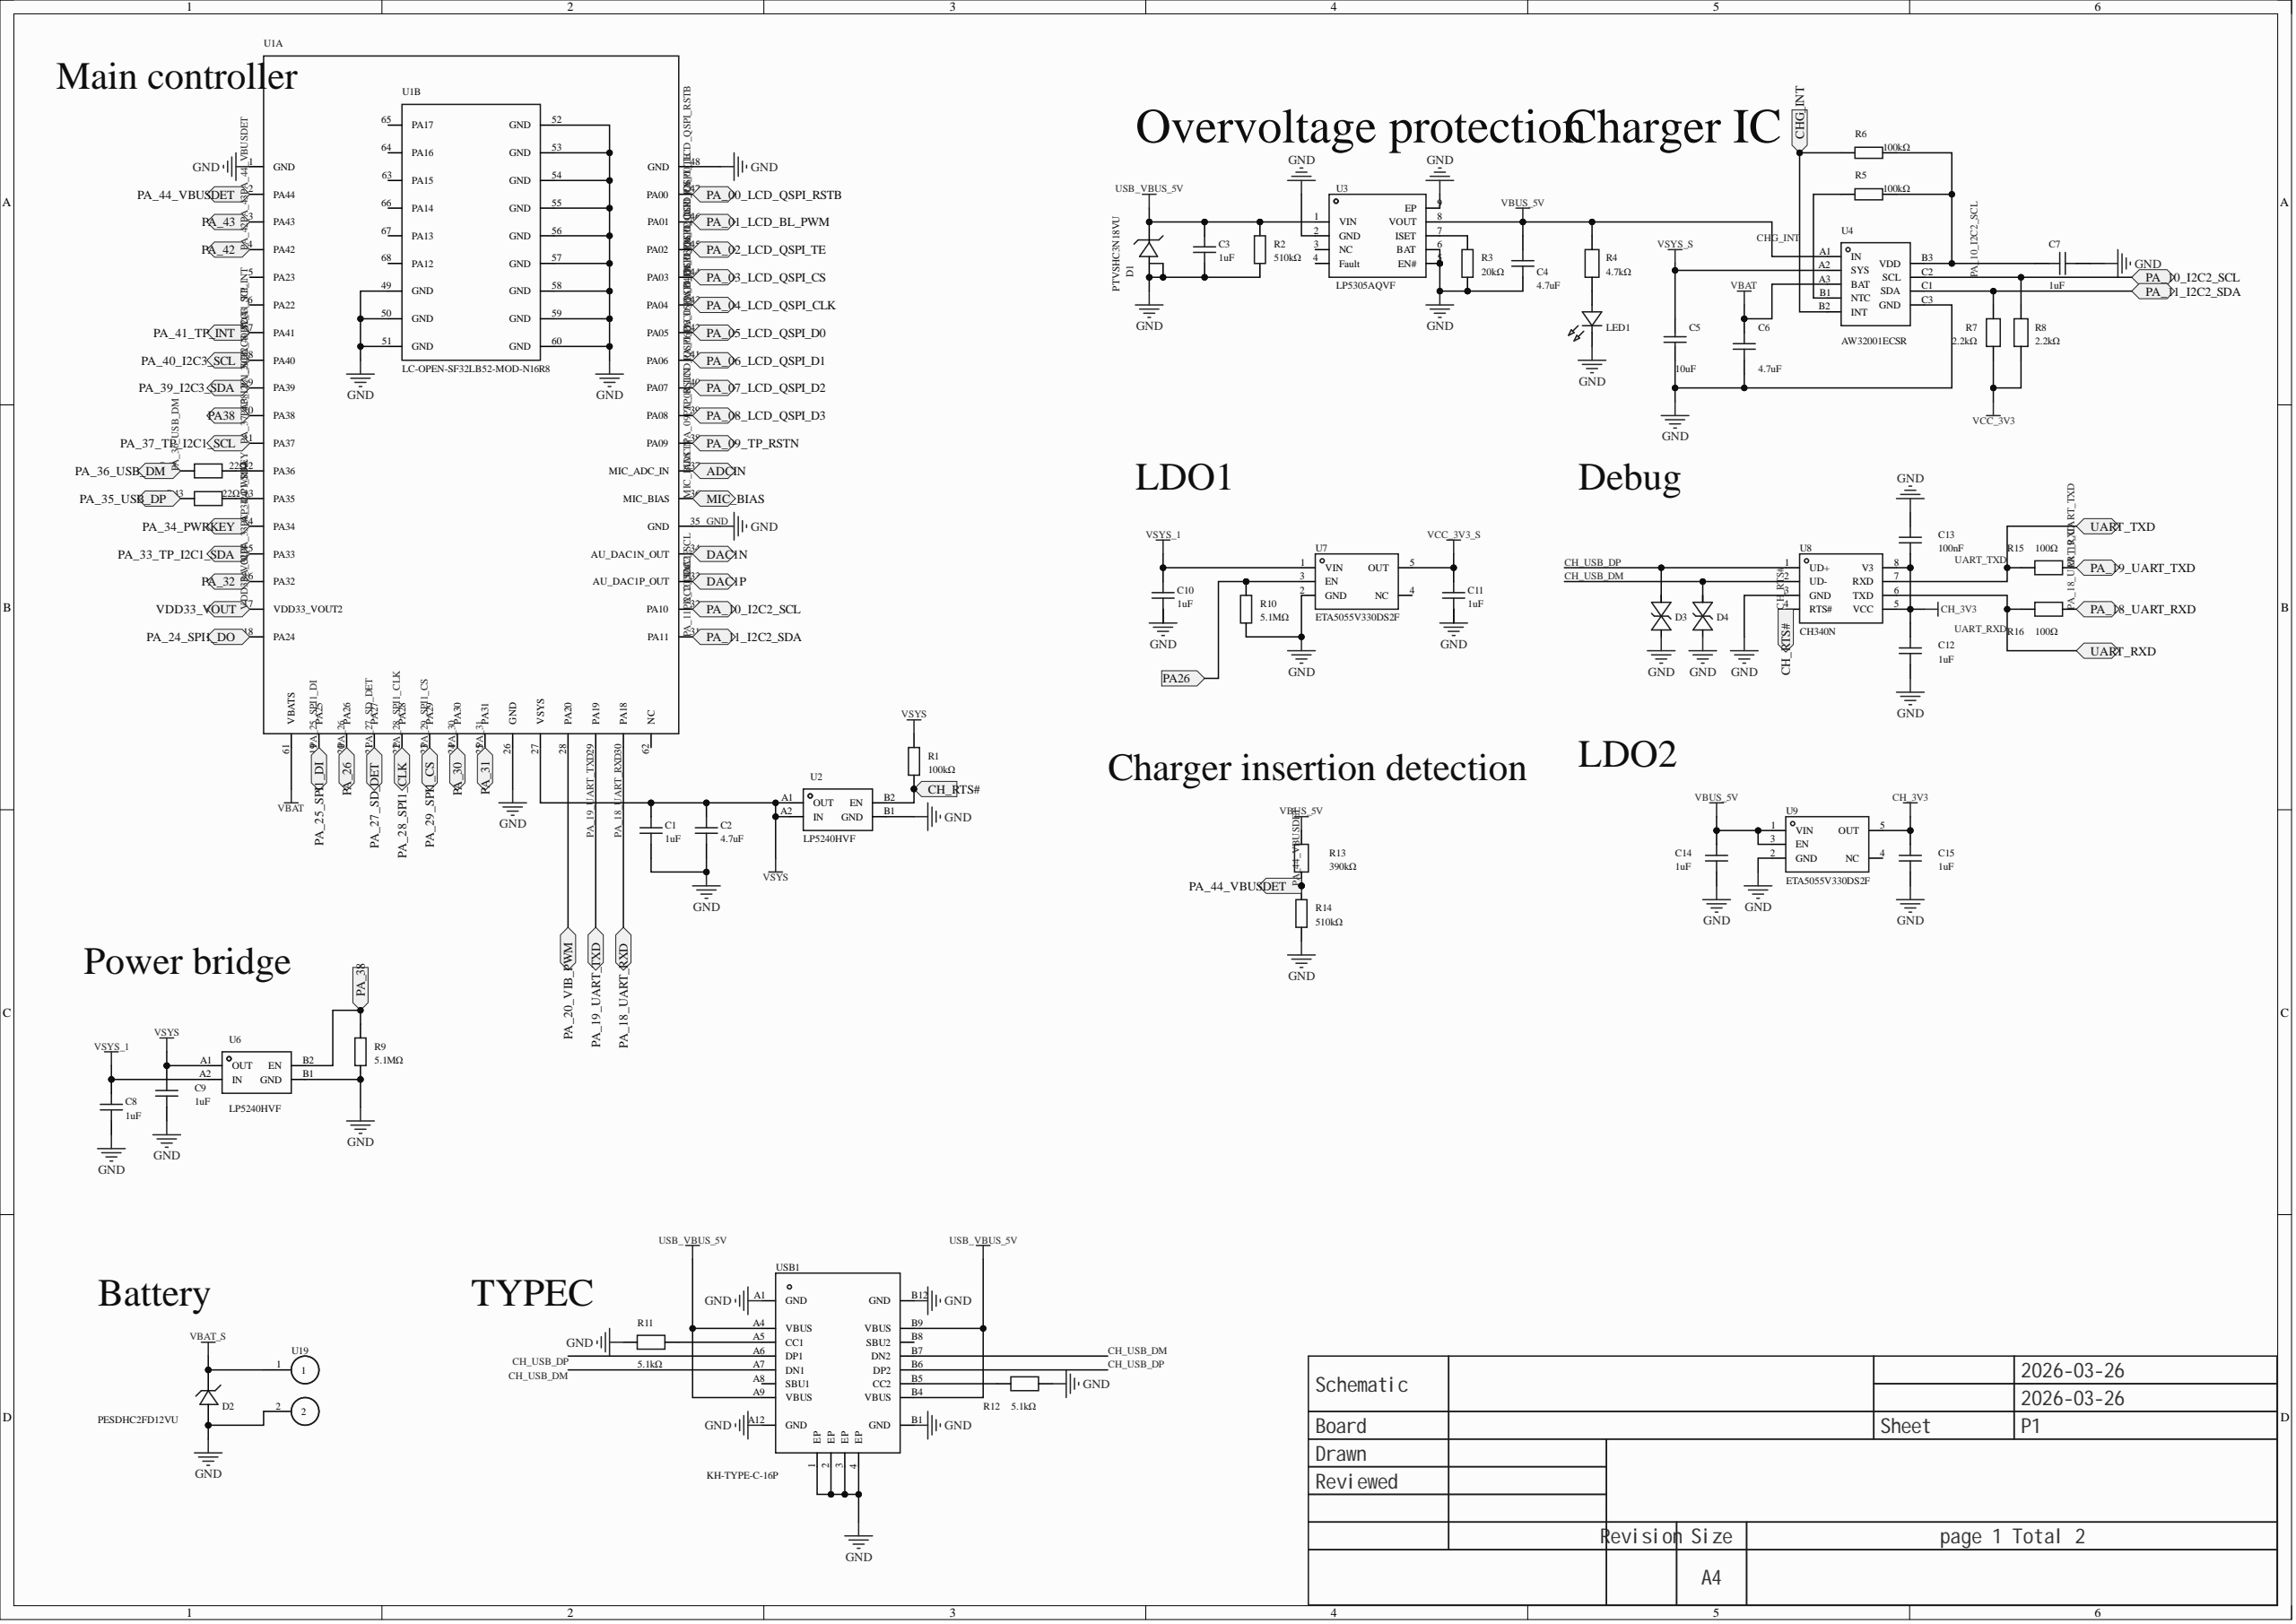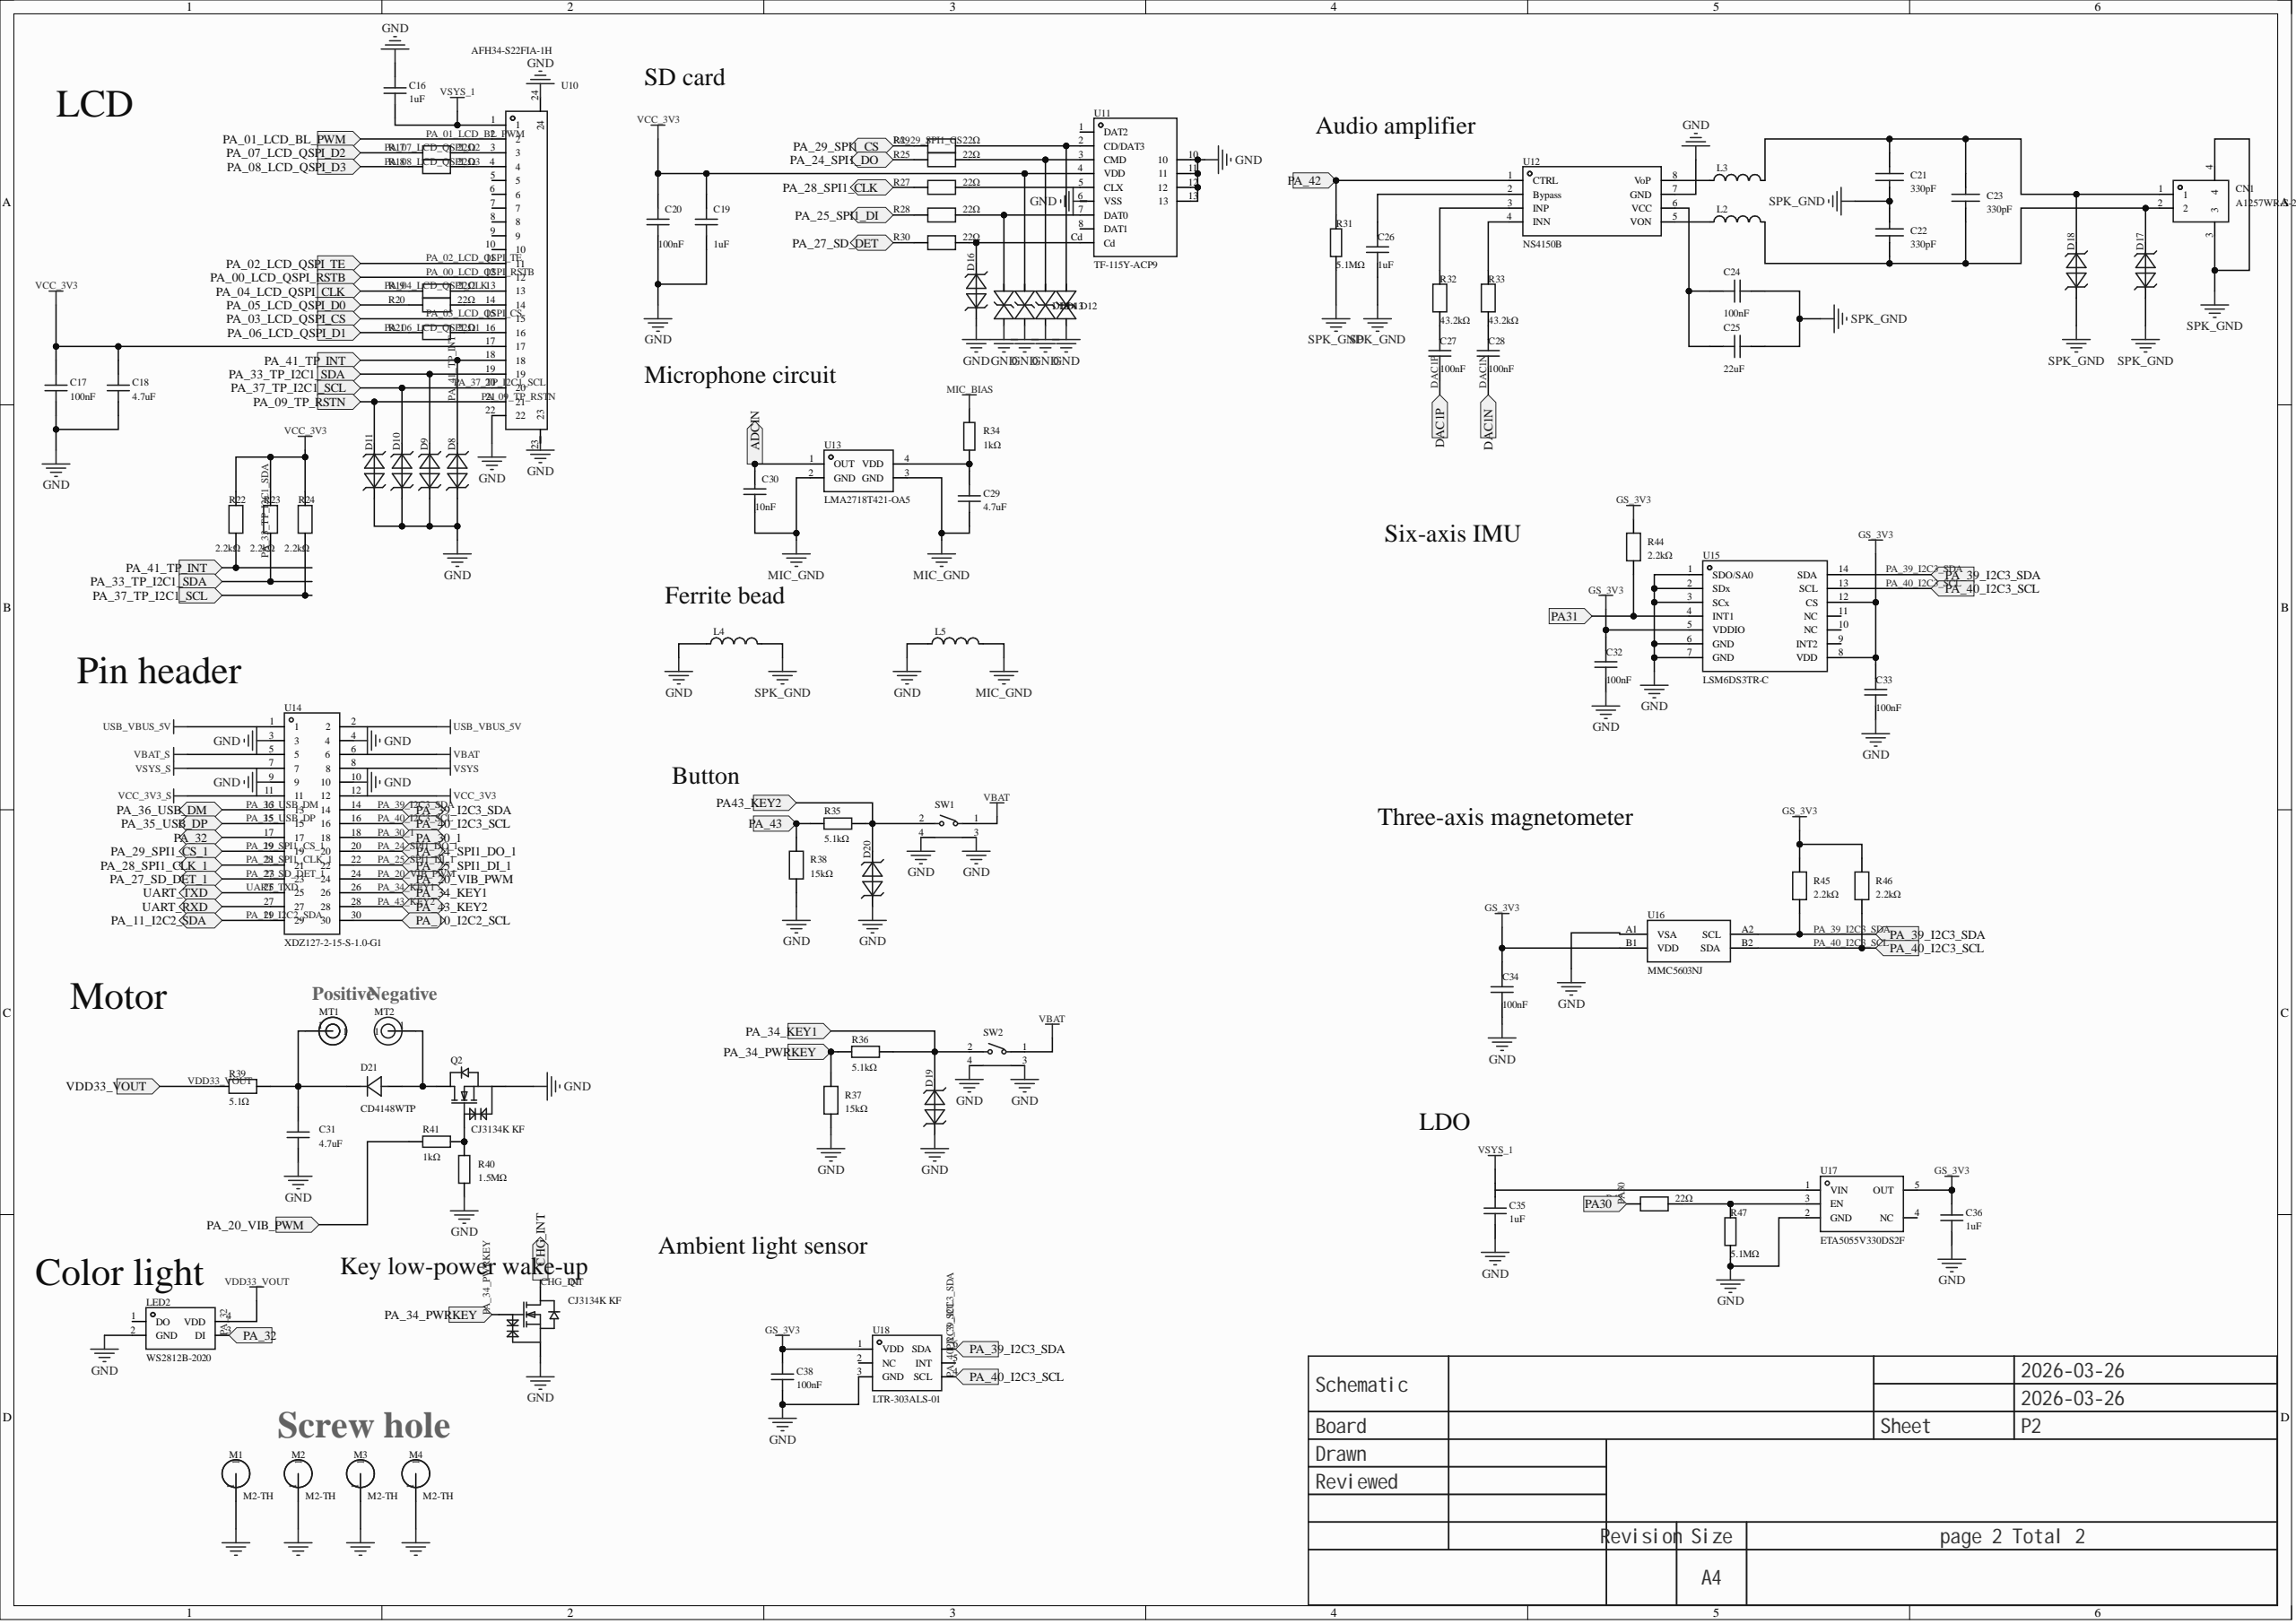Circuit board | Altium Designer | 138 parts | 94 nets
Bill of materials:
Comment,Description,Designator,Footprint,LibRef,Quantity
"1uF","Capacitance:1uF;Tolerance:±10%;Rated voltage:25V;Temperature coefficient:X5R;","C1, C3, C7, C8, C9, C10, C11, C12, C14, C15, C16, C19, C26, C35, C36","C0402","CL05A105KA5NQNC","15"
"4.7uF","Capacitance:4.7uF;Tolerance:±20%;Rated voltage:10V;Temperature coefficient:X5R;","C2, C4, C6, C18, C29, C31","C0402","CL05A475MP5NRNC","6"
"10uF","Capacitance:10uF;Tolerance:±20%;Rated voltage:6.3V;Temperature coefficient:X5R;","C5","C0402","CL05A106MQ5NUNC","1"
"100nF","Capacitance:100nF;Tolerance:±10%;Rated voltage:16V;Temperature coefficient:X7R;","C13, C17, C20, C24, C27, C28, C32, C33, C34, C38","C0402","CL05B104KO5NNNC","10"
"330pF","Capacitance:330pF;Tolerance:±5%;Rated voltage:50V;Temperature coefficient:C0G;","C21, C22, C23","C0402","CL05C331JB5NNNC","3"
"22uF","Capacitance:22uF;Tolerance:±20%;Rated voltage:6.3V;Temperature coefficient:X5R;","C25","C0402","GRM155R60J226ME11D","1"
"10nF","Capacitance:10nF;Tolerance:±10%;Rated voltage:50V;Temperature coefficient:X7R;","C30","C0402","CL05B103KB5NNNC","1"
"A1257WR-S-2P","Pin structure:1x2P;Pitch:1.25mm;Mounting:Horizontal;Reference series:GH;Total pins:2P;Rows:1;Pins per row:2;Row spacing:-;Rated current:1A;Contact material:Phosphor bronze;Contact plating:Tin;Operating temperature:-40℃~+105℃;","CN1","CONN-SMD_A1257WR-S-2P","A1257WR-S-2P","1"
"PTVSHC3N18VU","Reverse standoff voltage (Vrwm):18V;Clamping voltage:33V;Peak pulse current (Ipp):138A@8/20us;Peak pulse power (Ppp):4kW@8/20us;Breakdown voltage:20V;","D1","DFN-3_L2.0-W2.0-P1.30-BR","PTVSHC3N18VU","1"
"PESDHC2FD12VU","","D2","DFN1006-2L-RD","PESDHC2FD12VU","1"
"","Polarity:Bidirectional;Reverse standoff voltage (Vrwm):5V;Clamping voltage:40V;Peak pulse current (Ipp):-;Peak pulse power (Ppp):-;Breakdown voltage:-;","D3, D4, D12, D13, D14, D15","D0402-BI","KLXES15AAA1","6"
"ESD5451N","","D8, D9, D10, D11, D16, D17, D18, D19, D20","DFN1006-2L-BI","ESD5451N","9"
"CD4148WTP","Diode configuration:Discrete;Forward voltage (Vf):1.25V@100mA;DC reverse voltage (Vr):75V;Rectified current:150mA;Reverse recovery time (Trr):4ns;","D21","D0603-RD","CD4148WTP_C30584800","1"
"","Impedance@frequency:120Ω@100MHz;Tolerance:±25%;DC resistance (DCR):120mΩ;","L2, L3","L0402","PZ1005U121-1R0TF","2"
"","Impedance@frequency:0Ω@100MHz;DC resistance (DCR):100mΩ;","L4, L5","L0603","CBG160808U000T","2"
"","Lamp type:-;Emitted color:Emerald green;Forward voltage (Vf):2.6V~2.9V;Power:90mW;Forward current:30mA;Wavelength:520nm~525nm;Diode configuration:Discrete diode;Lens color:-;Color temperature:-;Luminous intensity:230mcd;Viewing angle:120°;Tape and reel:-;Operating temperature:-40℃~+85℃;","LED1","LED0603-RD_GREEN","F.0603.00025/P2-0603G1TS2-06T-002","1"
"WS2812B-2020","12mA, small size, high brightness, for small-pitch small-size products (note moisture sensitivity; see datasheet for details)","LED2","LED-SMD_4P-L2.0-W2.0-TL_WS2812B-2020","WS2812B-2020","1"
"M2-TH","","M1, M2, M3, M4","M2_TH_4_2.5MM","M2-TH","4"
"","","MT1, MT2","TP-3x2MM","TP_2x3MM","2"
"CJ3134K KF","Type:1 N-channel;Drain-source voltage (Vdss):20V;Continuous drain current (Id):750mA;On-resistance (RDS(on)):380mΩ@4.5V,650mA;Power dissipation (Pd):150mW;Threshold voltage (Vgs(th)):1.1V;","Q1, Q2","SOT-723_L1.2-W0.8-P0.40-LS1.2-BR","CJ3134K KF","2"
"100kΩ","Resistor type:Thick-film resistor;Resistance:100kΩ;Tolerance:±1%;Power:62.5mW;Operating voltage:50V;Temperature coefficient:±100ppm/?;","R1, R5, R6","R0402","0402WGF1003TCE","3"
"510kΩ","Resistor type:Thick-film resistor;Resistance:510kΩ;Tolerance:±1%;Power:62.5mW;Operating voltage:50V;Temperature coefficient:±100ppm/?;","R2, R14","R0402","0402WGF5103TCE","2"
"20kΩ","Resistor type:Thick-film resistor;Resistance:20kΩ;Tolerance:±1%;Power:62.5mW;Operating voltage:50V;Temperature coefficient:±100ppm/?;","R3","R0402","FRC0402F2002TS","1"
"4.7kΩ","Resistor type:Thick-film resistor;Resistance:4.7kΩ;Tolerance:±1%;Power:62.5mW;Operating voltage:50V;Temperature coefficient:±100ppm/?;","R4","R0402","FRC0402F4701TS","1"
"2.2kΩ","Resistor type:Thick-film resistor;Resistance:2.2kΩ;Tolerance:±1%;Power:62.5mW;Operating voltage:50V;Temperature coefficient:±100ppm/?;","R7, R8, R22, R23, R24, R44, R45, R46","R0402","FRC0402F2201TS","8"
"5.1MΩ","Resistor type:Thick-film resistor;Resistance:5.1MΩ;Tolerance:±1%;Power:62.5mW;Operating voltage:50V;Temperature coefficient:±100ppm/?;","R9, R10, R31, R47","R0402","0402WGF5104TCE","4"
"5.1kΩ","Resistor type:Thick-film resistor;Resistance:5.1kΩ;Tolerance:±1%;Power:62.5mW;Operating voltage:50V;Temperature coefficient:±100ppm/?;","R11, R12, R35, R36","R0402","FRC0402F5101TS, 0402WGF5101TCE","4"
"390kΩ","Resistor type:Thick-film resistor;Resistance:390kΩ;Tolerance:±1%;Power:62.5mW;Operating voltage:50V;Temperature coefficient:±100ppm/?;","R13","R0402","FRC0402F3903TS","1"
"100Ω","Resistor type:Thick-film resistor;Resistance:100Ω;Tolerance:±1%;Power:62.5mW;Operating voltage:50V;Temperature coefficient:±100ppm/?;","R15, R16","R0402","FRC0402F1000TS","2"
"22Ω","Resistor type:Thick-film resistor;Resistance:22Ω;Tolerance:±5%;Power:62.5mW;Operating voltage:50V;Temperature coefficient:±100ppm/?;","R17, R18, R19, R20, R21, R25, R27, R28, R29, R30, R42, R43, R48","R0402","FRC0402J220 TS","13"
"43.2kΩ","Resistor type:Thick-film resistor;Resistance:43.2kΩ;Tolerance:±1%;Power:62.5mW;Operating voltage:50V;Temperature coefficient:±100ppm/?;","R32, R33","R0402","FRC0402F4322TS","2"
"1kΩ","Resistor type:Thick-film resistor;Resistance:1kΩ;Tolerance:±1%;Power:62.5mW;Operating voltage:50V;Temperature coefficient:±100ppm/?;","R34, R41","R0402","RC0402FR-071KL","2"
"15kΩ","Resistor type:Thick-film resistor;Resistance:15kΩ;Tolerance:±1%;Power:62.5mW;Operating voltage:50V;Temperature coefficient:±100ppm/?;","R37, R38","R0402","FRC0402F1502TS","2"
"5.1Ω","Resistor type:Thick-film resistor;Resistance:5.1Ω;Tolerance:±1%;Power:62.5mW;Operating voltage:50V;Temperature coefficient:±200ppm/?;","R39","R0402","FRC0402F5R10TS","1"
"1.5MΩ","Resistance:1.5MΩ;Tolerance:±5%;Power:62.5mW;","R40","R0402","RCT021M5JLF","1"
"","Circuit structure:SPST;Button shape:Round button;Actuation force:1.8N;Mounting:Horizontal;Switch length:4.5mm;Switch width:2.2mm;Switch height:2.6mm;Bracket:Without bracket;Contact current:50mA;Rated voltage:12V;Lamp:None;Operating life:600万 cycles;","SW1, SW2","KEY-SMD_GT-TC191A-H026-L60","GT-TC191A-H026-L60","2"
"","Core chip:SF32LB525UC6 chip;Interface types:I2C; LCD; SPI; UART; USB; I2S; SDIO;Transmit power:19dBm;Communication distance:-;Receive sensitivity:-100dBm;","U1","COMM-SMD_L27.9-W18.0-P1.10_SF32LB52-MOD-1-N16R8","LC-OPEN-SF32LB52-MOD-N16R8","1"
"LP5240HVF","Type:Load switch;Channels:1;Input control logic:Active high;Max continuous current:1.5A;Operating voltage:1.2V~5.5V;On-resistance:50mΩ;","U2, U6","WLCSP-4_L0.8-W0.8-R2-C2-P0.40-BL","LP5240HVF","2"
"LP5305AQVF","Operating voltage:3.3V~26V;Max charge current:1A;Battery type:Lithium battery;Number of cells:1;","U3","DFN-8_L2.0-W2.0-P0.50-BL-EP","LP5305AQVF","1"
"AW32001ECSR","Operating voltage:4V~5.5V;Max charge current:500mA;Battery type:Lithium battery;Number of cells:1;","U4","WLCSP-9_L1.7-W1.7-R3-C3-P0.50-TL","AW32001ECSR","1"
"ETA5055V330DS2F","Output type:Fixed;Operating voltage:5.5V;Output voltage:3.3V;Output current:500mA;Power supply rejection ratio (PSRR):94dB@(1kHz);Output polarity:Positive;","U7, U9, U17","SOT-23-5_L2.9-W1.6-P0.95-LS2.8-BR","ETA5055V330DS2F","3"
"CH340N","Application function:USB to serial;USB version:USB 2.0;Channels:1;Data rate:2Mbps;","U8","SOP-8_L4.9-W3.9-P1.27-LS6.0-BL","CH340N","1"
"AFH34-S22FIA-1H","Locking feature:Flip type;Contact type:Dual-side contacts / top-bottom;Number of contacts:22P;Pitch:0.5mm;Mounting:Horizontal;","U10","FPC-SMD_22P-P0.50_JS_AFH34-S22FIA-1H","AFH34-S22FIA-1H","1"
"TF-115Y-ACP9","Card connection:Self-ejecting;Card type:MicroSD card (TF card);Connector type:Card socket;Max body height:-;Operating temperature:-25℃~+90℃;","U11","SIM-SMD_TF-115Y-BCP9","TF-115Y-ACP9","1"
"NS4150B","Amplifier type:Class D amplifier;Output power:3Wx1@4Ω;","U12","MSOP-8_L3.0-W3.0-P0.65-LS5.0-BL","NS4150B_C189961","1"
"LMA2718T421-OA5","Directivity:Omnidirectional;Signal-to-noise ratio:55dB;Sensitivity:-42dB;Impedance:300Ω;","U13","MIC-SMD_4P-L2.8-W1.9-P1.01-TL","LMA2718T421-OA5","1"
"XDZ127-2-15-S-1.0-G1","Pin structure:2x15P;Pitch:1.27mm;Round/square pin:Square pin;Mounting:Vertical;Rows:Double row;Total pin count:30P;Rated current:1A;Mating pin length:4mm;Plastic height:1mm;Operating temperature:-40℃~+105℃;Color:Black;","U14","HDR-SMD_30P-P1.27-V-M-R2-C15-LS5.5_1","XDZ127-2-15-S-1.0-G1","1"
"LSM6DS3TR-C","Sensor type:Accelerometer and gyroscope;Interface types:I2C; SPI;","U15","LGA-14_L3.0-W2.5-P0.50-TL","LSM6DS3TR-C","1"
"MMC5603NJ","The MMC5603NJ is a single-chip, complete three-axis anisotropic magnetoresistive (AMR) magnetic sensor with on-chip signal processing and an integrated digital bus (I²C Fast Mode and I3C interface). The device connects directly to a microprocessor without the need for an A/D converter or timing resources. It measures magnetic fields within ±30 gauss (G) full scale; in 20-bit operating mode, the resolution of each least significant bit (LSB) is up to 0.0625mG, with a total RMS noise level of 2mG, enabling compass heading accuracy of ±1°.","U16","FLIPCHIP-4_L0.8-W0.8-R2-C2-P0.40-TL","MMC5603NJ","1"
"LTR-303ALS-01","","U18","TDFN-6_L2.0-W2.0-P0.65-BL","LTR-303ALS-01","1"
"","","U19","焊盘","焊盘","1"
"KH-TYPE-C-16P","Connector type:Type-C;Protocol standard:-;Gender:Female;Mounting:Horizontal;Number of contacts:16P;Number of ports:1;Rated current - power:3A;Operating temperature:-40℃~+85℃;","USB1","USB-C-SMD_KH-TYPE-C-16P","KH-TYPE-C-16P","1"
Netlist (Protel format):
[
C1
C0402
1uF



]
[
C2
C0402
4.7uF



]
[
C3
C0402
1uF



]
[
C4
C0402
4.7uF



]
[
C5
C0402
10uF



]
[
C6
C0402
4.7uF



]
[
C7
C0402
1uF



]
[
C8
C0402
1uF



]
[
C9
C0402
1uF



]
[
C10
C0402
1uF



]
[
C11
C0402
1uF



]
[
C12
C0402
1uF



]
[
C13
C0402
100nF



]
[
C14
C0402
1uF



]
[
C15
C0402
1uF



]
[
C16
C0402
1uF



]
[
C17
C0402
100nF



]
[
C18
C0402
4.7uF



]
[
C19
C0402
1uF



]
[
C20
C0402
100nF



]
[
C21
C0402
330pF



]
[
C22
C0402
330pF



]
[
C23
C0402
330pF



]
[
C24
C0402
100nF



]
[
C25
C0402
22uF



]
[
C26
C0402
1uF



]
[
C27
C0402
100nF



]
[
C28
C0402
100nF



]
[
C29
C0402
4.7uF



]
[
C30
C0402
10nF



]
[
C31
C0402
4.7uF



]
[
C32
C0402
100nF



]
[
C33
C0402
100nF



]
[
C34
C0402
100nF



]
[
C35
C0402
1uF



]
[
C36
C0402
1uF



]
[
C38
C0402
100nF



]
[
CN1
CONN-SMD_A1257WR-S-2P
A1257WR-S-2P



]
[
D1
DFN-3_L2.0-W2.0-P1.30-BR
PTVSHC3N18VU



]
[
D2
DFN1006-2L-RD
PESDHC2FD12VU



]
[
D3
D0402-BI




]
[
D4
D0402-BI




]
[
D8
DFN1006-2L-BI
ESD5451N



]
[
D9
DFN1006-2L-BI
ESD5451N



]
[
D10
DFN1006-2L-BI
ESD5451N



]
[
D11
DFN1006-2L-BI
ESD5451N



]
[
D12
D0402-BI




]
[
D13
D0402-BI




]
[
D14
D0402-BI




]
[
D15
D0402-BI




]
[
D16
DFN1006-2L-BI
ESD5451N



]
[
D17
DFN1006-2L-BI
ESD5451N



]
[
D18
DFN1006-2L-BI
ESD5451N



]
[
D19
DFN1006-2L-BI
ESD5451N



]
[
D20
DFN1006-2L-BI
ESD5451N



]
[
D21
D0603-RD
CD4148WTP



]
[
L2
L0402




]
[
L3
L0402




]
[
L4
L0603




]
[
L5
L0603




]
[
LED1
LED0603-RD_GREEN




]
[
LED2
LED-SMD_4P-L2.0-W2.0-TL_WS2812B-2020
WS2812B-2020



]
[
M1
M2_TH_4_2.5MM
M2-TH



]
[
M2
M2_TH_4_2.5MM
M2-TH



]
[
M3
M2_TH_4_2.5MM
M2-TH



]
[
M4
M2_TH_4_2.5MM
M2-TH



]
[
MT1
TP-3x2MM




]
[
MT2
TP-3x2MM




]
[
Q1
SOT-723_L1.2-W0.8-P0.40-LS1.2-BR
CJ3134K KF



]
[
Q2
SOT-723_L1.2-W0.8-P0.40-LS1.2-BR
CJ3134K KF



]
[
R1
R0402
100kΩ



]
[
R2
R0402
510kΩ



]
[
R3
R0402
20kΩ



]
[
R4
R0402
4.7kΩ



]
[
R5
R0402
100kΩ



]
[
R6
R0402
100kΩ



]
[
R7
R0402
2.2kΩ



]
[
R8
R0402
2.2kΩ



]
[
R9
R0402
5.1MΩ



]
[
R10
R0402
5.1MΩ



]
[
R11
R0402
5.1kΩ



]
[
R12
R0402
5.1kΩ



]
[
R13
R0402
390kΩ



]
[
R14
R0402
510kΩ



]
[
R15
R0402
100Ω



]
[
R16
R0402
100Ω



]
[
R17
R0402
22Ω



]
[
R18
R0402
22Ω



]
[
R19
R0402
22Ω



]
[
R20
R0402
22Ω



]
[
R21
R0402
22Ω



]
[
R22
R0402
2.2kΩ



]
[
R23
R0402
2.2kΩ



]
[
R24
R0402
2.2kΩ



]
[
R25
R0402
22Ω



]
[
R27
R0402
22Ω



]
[
R28
R0402
22Ω



]
[
R29
R0402
22Ω



]
[
R30
R0402
22Ω



]
[
R31
R0402
5.1MΩ



]
[
R32
R0402
43.2kΩ



]
[
R33
R0402
43.2kΩ



]
[
R34
R0402
1kΩ



]
[
R35
R0402
5.1kΩ



]
[
R36
R0402
5.1kΩ



]
[
R37
R0402
15kΩ



]
[
R38
R0402
15kΩ



]
[
R39
R0402
5.1Ω



]
[
R40
R0402
1.5MΩ



]
[
R41
R0402
1kΩ



]
[
R42
R0402
22Ω



]
[
R43
R0402
22Ω



]
[
R44
R0402
2.2kΩ



]
[
R45
R0402
2.2kΩ



]
[
R46
R0402
2.2kΩ



]
[
R47
R0402
5.1MΩ



]
[
R48
R0402
22Ω



]
[
SW1
KEY-SMD_GT-TC191A-H026-L60




]
[
SW2
KEY-SMD_GT-TC191A-H026-L60




]
[
U1
COMM-SMD_L27.9-W18.0-P1.10_SF32LB52-MOD-1-N16R8




]
[
U2
WLCSP-4_L0.8-W0.8-R2-C2-P0.40-BL
LP5240HVF



]
[
U3
DFN-8_L2.0-W2.0-P0.50-BL-EP
LP5305AQVF



]
[
U4
WLCSP-9_L1.7-W1.7-R3-C3-P0.50-TL
AW32001ECSR



]
[
U6
WLCSP-4_L0.8-W0.8-R2-C2-P0.40-BL
LP5240HVF



]
[
U7
SOT-23-5_L2.9-W1.6-P0.95-LS2.8-BR
ETA5055V330DS2F



]
[
U8
SOP-8_L4.9-W3.9-P1.27-LS6.0-BL
CH340N



]
[
U9
SOT-23-5_L2.9-W1.6-P0.95-LS2.8-BR
ETA5055V330DS2F



]
[
U10
FPC-SMD_22P-P0.50_JS_AFH34-S22FIA-1H
AFH34-S22FIA-1H



]
[
U11
SIM-SMD_TF-115Y-BCP9
TF-115Y-ACP9



]
[
U12
MSOP-8_L3.0-W3.0-P0.65-LS5.0-BL
NS4150B



]
[
U13
MIC-SMD_4P-L2.8-W1.9-P1.01-TL
LMA2718T421-OA5



]
[
U14
HDR-SMD_30P-P1.27-V-M-R2-C15-LS5.5_1
XDZ127-2-15-S-1.0-G1



]
[
U15
LGA-14_L3.0-W2.5-P0.50-TL
LSM6DS3TR-C



]
[
U16
FLIPCHIP-4_L0.8-W0.8-R2-C2-P0.40-TL
MMC5603NJ



]
[
U17
SOT-23-5_L2.9-W1.6-P0.95-LS2.8-BR
ETA5055V330DS2F



]
[
U18
TDFN-6_L2.0-W2.0-P0.65-BL
LTR-303ALS-01



]
[
U19
焊盘




]
[
USB1
USB-C-SMD_KH-TYPE-C-16P
KH-TYPE-C-16P



]
(
VSYS_S
C5-1
U4-A2
U14-7
)
(
VSYS_1
C8-2
C10-2
C16-1
C35-2
U6-A2
U7-1
U10-1
)
(
VSYS
C1-2
C2-2
C9-2
R1-2
U1-27
U2-A1
U2-A2
U6-A1
U14-8
)
(
VDD33_VOUT
LED2-4
R39-1
U1-17
)
(
VCC_3V3_S
C11-2
U7-5
U14-11
)
(
VCC_3V3
C17-2
C18-2
C19-2
C20-2
D14-2
R7-1
R8-1
R22-2
R23-2
R24-2
U10-17
U11-4
U14-12
)
(
VBUS_5V
C4-2
C14-2
R4-2
R13-2
U3-8
U4-A1
U9-1
U9-3
)
(
VBAT_S
D2-1
U14-5
U19-1
)
(
VBAT
C6-1
SW1-1
SW2-1
U1-61
U4-A3
U14-6
)
(
USB_VBUS_5V
C3-2
D1-3
R2-2
U3-1
U14-1
U14-2
USB1-A4
USB1-A9
USB1-B4
USB1-B9
)
(
UART_TXD
R15-1
U8-7
U14-25
)
(
UART_RXD
R16-1
U8-6
U14-27
)
(
SPK_GND
C21-1
C22-2
C24-1
C25-1
C26-1
CN1-3
CN1-4
D17-1
D18-1
L4-2
R31-1
)
(
PA_44_VBUSDET
R13-1
R14-2
U1-2
)
(
PA_43
R35-1
R38-2
U1-3
)
(
PA_42
R31-2
U1-4
U12-1
)
(
PA_41_TP_INT
D8-2
R22-1
U1-7
U10-18
)
(
PA_40_I2C3_SCL
R46-1
U1-8
U14-16
U15-13
U16-B2
U18-4
)
(
PA_39_I2C3_SDA
R45-1
U1-9
U14-14
U15-14
U16-A2
U18-6
)
(
PA_37_TP_I2C1_SCL
D10-2
R24-1
U1-11
U10-20
)
(
PA_36_USB_DM
R42-1
U14-13
)
(
PA_35_USB_DP
R43-2
U14-15
)
(
PA_34_PWRKEY
Q1-1
R36-1
R37-2
U1-14
)
(
PA_34_KEY1
D19-2
R36-2
SW2-2
U14-26
)
(
PA_33_TP_I2C1_SDA
D9-2
R23-1
U1-15
U10-19
)
(
PA_32
LED2-3
U1-16
U14-17
)
(
PA_29_SPI1_CS
R29-1
U1-23
)
(
PA_28_SPI1_CLK
R27-1
U1-22
)
(
PA_27_SD_DET
R30-1
U1-21
)
(
PA_25_SPI1_DI
R28-1
U1-19
)
(
PA_20_VIB_PWM
R41-2
U1-28
U14-24
)
(
PA_19_UART_TXD
R15-2
U1-29
)
(
PA_18_UART_RXD
R16-2
U1-30
)
(
PA_11_I2C2_SDA
R7-2
U1-31
U4-C1
U14-29
)
(
PA_10_I2C2_SCL
R8-2
U1-32
U4-C2
U14-30
)
(
PA_09_TP_RSTN
D11-2
U1-38
U10-21
)
(
PA_08_LCD_QSPI_D3
R18-1
U1-39
)
(
PA_07_LCD_QSPI_D2
R17-1
U1-40
)
(
PA_06_LCD_QSPI_D1
R21-1
U1-41
)
(
PA_05_LCD_QSPI_D0
R20-1
U1-42
)
(
PA_04_LCD_QSPI_CLK
R19-1
U1-43
)
(
PA_03_LCD_QSPI_CS
U1-44
U10-15
)
(
PA_02_LCD_QSPI_TE
U1-45
U10-11
)
(
PA_01_LCD_BL_PWM
U1-46
U10-2
)
(
PA_00_LCD_QSPI_RSTB
U1-47
U10-12
)
(
NetR47_2
R47-2
R48-2
U17-3
)
(
NetR44_1
R44-1
U15-4
)
(
NetR43_1
R43-1
U1-13
)
(
NetR42_2
R42-2
U1-12
)
(
NetR33_2
R33-2
U12-4
)
(
NetR32_2
R32-2
U12-3
)
(
NetR27_2
R27-2
U11-5
)
(
NetR25_1
R25-1
U1-18
)
(
NetR21_2
R21-2
U10-16
)
(
NetR20_2
R20-2
U10-14
)
(
NetR19_2
R19-2
U10-13
)
(
NetR18_2
R18-2
U10-4
)
(
NetR17_2
R17-2
U10-3
)
(
NetR12_1
R12-1
USB1-B5
)
(
NetR11_2
R11-2
USB1-A5
)
(
NetR10_2
R10-2
U7-3
)
(
NetR9_2
R9-2
U6-B2
)
(
NetR5_2
R5-2
U4-B1
)
(
NetR3_2
R3-2
U3-7
)
(
NetQ2_1
Q2-1
R40-2
R41-1
)
(
NetLED1_2
LED1-2
R4-1
)
(
NetL3_1
L3-1
U12-8
)
(
NetL2_1
L2-1
U12-5
)
(
NetD21_2
D21-2
MT2-1
Q2-3
)
(
NetD20_2
D20-2
R35-2
SW1-2
)
(
NetD16_2
D16-2
R30-2
U11-Cd
)
(
NetD15_2
D15-2
R28-2
U11-7
)
(
NetD13_2
D13-2
R25-2
U11-3
)
(
NetD12_2
D12-2
R29-2
U11-2
)
(
NetC31_2
C31-2
D21-1
MT1-1
R39-2
)
(
NetC29_2
C29-2
R34-1
U13-4
)
(
NetC28_1
C28-1
R33-1
)
(
NetC27_1
C27-1
R32-1
)
(
NetC26_2
C26-2
U12-2
)
(
NetC24_2
C24-2
C25-2
U12-6
)
(
NetC22_1
C22-1
C23-1
CN1-2
D17-2
L2-2
)
(
NetC21_2
C21-2
C23-2
CN1-1
D18-2
L3-2
)
(
NetC7_1
C7-1
R5-1
R6-1
U4-B3
)
(
MIC_GND
C29-1
C30-1
L5-2
U13-2
U13-3
)
(
GS_3V3
C32-1
C33-1
C34-1
C36-2
C38-2
R44-2
R45-2
R46-2
U15-5
U15-8
U15-12
U16-B1
U17-5
U18-1
)
(
GND
C1-1
C2-1
C3-1
C4-1
C5-2
C6-2
C7-2
C8-1
C9-1
C10-1
C11-1
C12-1
C13-2
C14-1
C15-1
C16-2
C17-1
C18-1
C19-1
C20-1
C31-1
C32-2
C33-2
C34-2
C35-1
C36-1
C38-1
D1-1
D1-2
D2-2
D3-1
D4-1
D8-1
D9-1
D10-1
D11-1
D12-1
D13-1
D14-1
D15-1
D16-1
D19-1
D20-1
L4-1
L5-1
LED1-1
LED2-2
M1-1
M2-1
M3-1
M4-1
Q1-2
Q2-2
R2-1
R3-1
R9-1
R10-1
R11-1
R12-2
R14-1
R37-1
R38-1
R40-1
R47-1
SW1-3
SW1-4
SW2-3
SW2-4
U1-1
U1-26
U1-35
U1-48
U1-49
U1-50
U1-51
U1-52
U1-53
U1-54
U1-55
U1-56
U1-57
U1-58
U1-59
U1-60
U2-B1
U3-2
U3-5
U3-6
U3-9
U4-C3
U6-B1
U7-2
U8-3
U9-2
U10-22
U10-23
U10-24
U11-6
U11-10
U11-11
U11-12
U11-13
U12-7
U14-3
U14-4
U14-9
U14-10
U15-1
U15-2
U15-3
U15-6
U15-7
U16-A1
U17-2
U18-3
U19-2
USB1-1
USB1-2
USB1-3
USB1-4
USB1-A1
USB1-A12
USB1-B1
USB1-B12
)
(
DAC1P
C27-2
U1-33
)
(
DAC1N
C28-2
U1-34
)
(
CHG_INT
Q1-3
R6-2
U4-B2
)
(
CH_USB_DP
D3-2
U8-1
USB1-A6
USB1-B6
)
(
CH_USB_DM
D4-2
U8-2
USB1-A7
USB1-B7
)
(
CH_RTS#
R1-1
U2-B2
U8-4
)
(
CH_3V3
C12-2
C13-1
C15-2
U8-5
U8-8
U9-5
)
(
ADCIN
C30-2
U1-37
U13-1
)